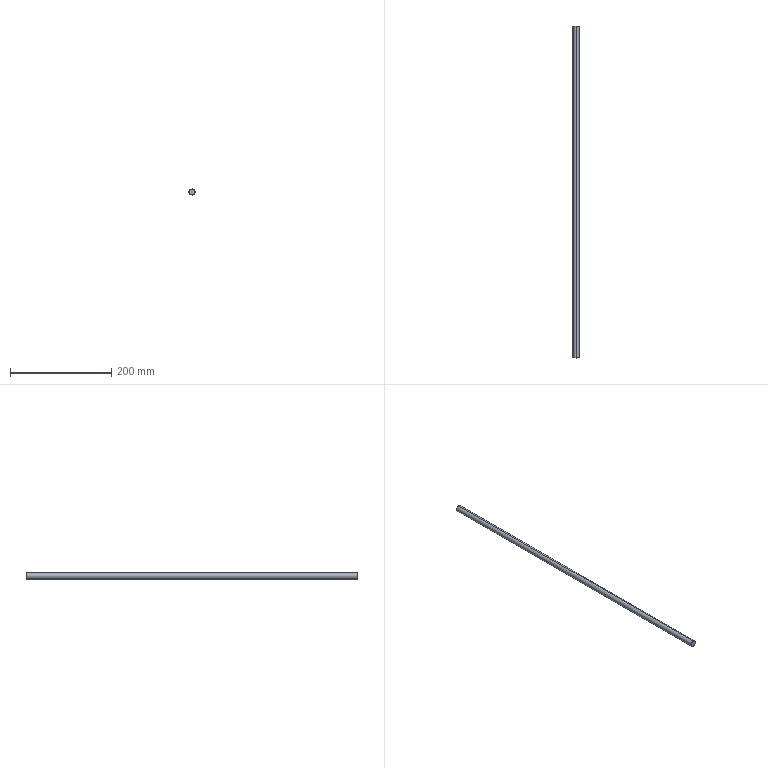Part | SolidWorks | features BaseBody 1 | 1 solid | 8 faces | box 12 x 656 x 12 mm | volume 74183 mm3 | cone 4 | cylinder 2 | plane 2 | commonest cylinder face diameters 12 x2
STEP:
#1=CARTESIAN_POINT('',(0.,0.,-5.5));
#2=VERTEX_POINT('',#1);
#3=CARTESIAN_POINT('',(0.,0.,5.5));
#4=VERTEX_POINT('',#3);
#5=CARTESIAN_POINT('',(0.,0.,0.));
#6=DIRECTION('',(0.,-1.,0.));
#7=DIRECTION('',(0.,0.,1.));
#8=AXIS2_PLACEMENT_3D('',#5,#6,#7);
#9=CIRCLE('',#8,5.5);
#10=EDGE_CURVE('',#2,#4,#9,.T.);
#11=ORIENTED_EDGE('',*,*,#10,.F.);
#12=CARTESIAN_POINT('',(0.,0.5,-6.));
#13=VERTEX_POINT('',#12);
#14=CARTESIAN_POINT('',(0.,0.5,-6.));
#15=DIRECTION('',(0.,0.7071,-0.7071));
#16=VECTOR('',#15,1000.);
#17=LINE('',#14,#16);
#18=EDGE_CURVE('',#2,#13,#17,.T.);
#19=ORIENTED_EDGE('',*,*,#18,.T.);
#20=CARTESIAN_POINT('',(0.,0.5,6.));
#21=VERTEX_POINT('',#20);
#22=CARTESIAN_POINT('',(0.,0.5,0.));
#23=DIRECTION('',(0.,1.,0.));
#24=DIRECTION('',(0.,0.,1.));
#25=AXIS2_PLACEMENT_3D('',#22,#23,#24);
#26=CIRCLE('',#25,6.);
#27=EDGE_CURVE('',#21,#13,#26,.T.);
#28=ORIENTED_EDGE('',*,*,#27,.F.);
#29=CARTESIAN_POINT('',(0.,0.5,6.));
#30=DIRECTION('',(0.,0.7071,0.7071));
#31=VECTOR('',#30,1000.);
#32=LINE('',#29,#31);
#33=EDGE_CURVE('',#4,#21,#32,.T.);
#34=ORIENTED_EDGE('',*,*,#33,.F.);
#35=EDGE_LOOP('',(#11,#19,#28,#34));
#36=FACE_OUTER_BOUND('',#35,.T.);
#37=CARTESIAN_POINT('',(0.,0.5,0.));
#38=DIRECTION('',(0.,1.,0.));
#39=DIRECTION('',(0.,0.,1.));
#40=AXIS2_PLACEMENT_3D('',#37,#38,#39);
#41=CONICAL_SURFACE('',#40,6.,0.7854);
#42=ADVANCED_FACE('',(#36),#41,.T.);
#43=CARTESIAN_POINT('',(0.,656.,5.5));
#44=VERTEX_POINT('',#43);
#45=CARTESIAN_POINT('',(0.,656.,-5.5));
#46=VERTEX_POINT('',#45);
#47=CARTESIAN_POINT('',(0.,656.,0.));
#48=DIRECTION('',(0.,1.,0.));
#49=DIRECTION('',(0.,0.,1.));
#50=AXIS2_PLACEMENT_3D('',#47,#48,#49);
#51=CIRCLE('',#50,5.5);
#52=EDGE_CURVE('',#44,#46,#51,.T.);
#53=ORIENTED_EDGE('',*,*,#52,.F.);
#54=CARTESIAN_POINT('',(0.,655.5,6.));
#55=VERTEX_POINT('',#54);
#56=CARTESIAN_POINT('',(0.,656.,5.5));
#57=DIRECTION('',(0.,-0.7071,0.7071));
#58=VECTOR('',#57,1000.);
#59=LINE('',#56,#58);
#60=EDGE_CURVE('',#44,#55,#59,.T.);
#61=ORIENTED_EDGE('',*,*,#60,.T.);
#62=CARTESIAN_POINT('',(0.,655.5,-6.));
#63=VERTEX_POINT('',#62);
#64=CARTESIAN_POINT('',(0.,655.5,0.));
#65=DIRECTION('',(0.,-1.,0.));
#66=DIRECTION('',(0.,0.,1.));
#67=AXIS2_PLACEMENT_3D('',#64,#65,#66);
#68=CIRCLE('',#67,6.);
#69=EDGE_CURVE('',#63,#55,#68,.T.);
#70=ORIENTED_EDGE('',*,*,#69,.F.);
#71=CARTESIAN_POINT('',(0.,656.,-5.5));
#72=DIRECTION('',(0.,-0.7071,-0.7071));
#73=VECTOR('',#72,1000.);
#74=LINE('',#71,#73);
#75=EDGE_CURVE('',#46,#63,#74,.T.);
#76=ORIENTED_EDGE('',*,*,#75,.F.);
#77=EDGE_LOOP('',(#53,#61,#70,#76));
#78=FACE_OUTER_BOUND('',#77,.T.);
#79=CARTESIAN_POINT('',(0.,656.,0.));
#80=DIRECTION('',(0.,-1.,0.));
#81=DIRECTION('',(0.,0.,-1.));
#82=AXIS2_PLACEMENT_3D('',#79,#80,#81);
#83=CONICAL_SURFACE('',#82,5.5,0.7854);
#84=ADVANCED_FACE('',(#78),#83,.T.);
#85=ORIENTED_EDGE('',*,*,#69,.T.);
#86=CARTESIAN_POINT('',(0.,656.,6.));
#87=DIRECTION('',(0.,-1.,0.));
#88=VECTOR('',#87,1000.);
#89=LINE('',#86,#88);
#90=EDGE_CURVE('',#55,#21,#89,.T.);
#91=ORIENTED_EDGE('',*,*,#90,.T.);
#92=ORIENTED_EDGE('',*,*,#27,.T.);
#93=CARTESIAN_POINT('',(0.,656.,-6.));
#94=DIRECTION('',(0.,-1.,0.));
#95=VECTOR('',#94,1000.);
#96=LINE('',#93,#95);
#97=EDGE_CURVE('',#63,#13,#96,.T.);
#98=ORIENTED_EDGE('',*,*,#97,.F.);
#99=EDGE_LOOP('',(#85,#91,#92,#98));
#100=FACE_OUTER_BOUND('',#99,.T.);
#101=CARTESIAN_POINT('',(0.,656.,0.));
#102=DIRECTION('',(0.,-1.,0.));
#103=DIRECTION('',(0.,0.,-1.));
#104=AXIS2_PLACEMENT_3D('',#101,#102,#103);
#105=CYLINDRICAL_SURFACE('',#104,6.);
#106=ADVANCED_FACE('',(#100),#105,.T.);
#107=CARTESIAN_POINT('',(0.,0.,0.));
#108=DIRECTION('',(0.,-1.,0.));
#109=DIRECTION('',(0.,0.,1.));
#110=AXIS2_PLACEMENT_3D('',#107,#108,#109);
#111=CIRCLE('',#110,5.5);
#112=EDGE_CURVE('',#4,#2,#111,.T.);
#113=ORIENTED_EDGE('',*,*,#112,.T.);
#114=ORIENTED_EDGE('',*,*,#10,.T.);
#115=EDGE_LOOP('',(#113,#114));
#116=FACE_OUTER_BOUND('',#115,.T.);
#117=CARTESIAN_POINT('',(0.,0.,0.));
#118=DIRECTION('',(0.,1.,0.));
#119=DIRECTION('',(1.,0.,0.));
#120=AXIS2_PLACEMENT_3D('',#117,#118,#119);
#121=PLANE('',#120);
#122=ADVANCED_FACE('',(#116),#121,.F.);
#123=CARTESIAN_POINT('',(0.,656.,0.));
#124=DIRECTION('',(0.,1.,0.));
#125=DIRECTION('',(0.,0.,1.));
#126=AXIS2_PLACEMENT_3D('',#123,#124,#125);
#127=CIRCLE('',#126,5.5);
#128=EDGE_CURVE('',#46,#44,#127,.T.);
#129=ORIENTED_EDGE('',*,*,#128,.T.);
#130=ORIENTED_EDGE('',*,*,#52,.T.);
#131=EDGE_LOOP('',(#129,#130));
#132=FACE_OUTER_BOUND('',#131,.T.);
#133=CARTESIAN_POINT('',(0.,656.,0.));
#134=DIRECTION('',(0.,1.,0.));
#135=DIRECTION('',(1.,0.,0.));
#136=AXIS2_PLACEMENT_3D('',#133,#134,#135);
#137=PLANE('',#136);
#138=ADVANCED_FACE('',(#132),#137,.T.);
#139=ORIENTED_EDGE('',*,*,#90,.F.);
#140=CARTESIAN_POINT('',(0.,655.5,0.));
#141=DIRECTION('',(0.,-1.,0.));
#142=DIRECTION('',(0.,0.,1.));
#143=AXIS2_PLACEMENT_3D('',#140,#141,#142);
#144=CIRCLE('',#143,6.);
#145=EDGE_CURVE('',#55,#63,#144,.T.);
#146=ORIENTED_EDGE('',*,*,#145,.T.);
#147=ORIENTED_EDGE('',*,*,#97,.T.);
#148=CARTESIAN_POINT('',(0.,0.5,0.));
#149=DIRECTION('',(0.,1.,0.));
#150=DIRECTION('',(0.,0.,1.));
#151=AXIS2_PLACEMENT_3D('',#148,#149,#150);
#152=CIRCLE('',#151,6.);
#153=EDGE_CURVE('',#13,#21,#152,.T.);
#154=ORIENTED_EDGE('',*,*,#153,.T.);
#155=EDGE_LOOP('',(#139,#146,#147,#154));
#156=FACE_OUTER_BOUND('',#155,.T.);
#157=CARTESIAN_POINT('',(0.,656.,0.));
#158=DIRECTION('',(0.,-1.,0.));
#159=DIRECTION('',(0.,0.,-1.));
#160=AXIS2_PLACEMENT_3D('',#157,#158,#159);
#161=CYLINDRICAL_SURFACE('',#160,6.);
#162=ADVANCED_FACE('',(#156),#161,.T.);
#163=ORIENTED_EDGE('',*,*,#60,.F.);
#164=ORIENTED_EDGE('',*,*,#128,.F.);
#165=ORIENTED_EDGE('',*,*,#75,.T.);
#166=ORIENTED_EDGE('',*,*,#145,.F.);
#167=EDGE_LOOP('',(#163,#164,#165,#166));
#168=FACE_OUTER_BOUND('',#167,.T.);
#169=CARTESIAN_POINT('',(0.,656.,0.));
#170=DIRECTION('',(0.,-1.,0.));
#171=DIRECTION('',(0.,0.,-1.));
#172=AXIS2_PLACEMENT_3D('',#169,#170,#171);
#173=CONICAL_SURFACE('',#172,5.5,0.7854);
#174=ADVANCED_FACE('',(#168),#173,.T.);
#175=ORIENTED_EDGE('',*,*,#18,.F.);
#176=ORIENTED_EDGE('',*,*,#112,.F.);
#177=ORIENTED_EDGE('',*,*,#33,.T.);
#178=ORIENTED_EDGE('',*,*,#153,.F.);
#179=EDGE_LOOP('',(#175,#176,#177,#178));
#180=FACE_OUTER_BOUND('',#179,.T.);
#181=CARTESIAN_POINT('',(0.,0.5,0.));
#182=DIRECTION('',(0.,1.,0.));
#183=DIRECTION('',(0.,0.,1.));
#184=AXIS2_PLACEMENT_3D('',#181,#182,#183);
#185=CONICAL_SURFACE('',#184,6.,0.7854);
#186=ADVANCED_FACE('',(#180),#185,.T.);
#187=CLOSED_SHELL('',(#42,#84,#106,#122,#138,#162,#174,#186));
#188=MANIFOLD_SOLID_BREP('',#187);
#189=CARTESIAN_POINT('',(0.,0.,0.));
#190=DIRECTION('',(0.,0.,1.));
#191=DIRECTION('',(1.,0.,0.));
#192=AXIS2_PLACEMENT_3D('',#189,#190,#191);
#193=(LENGTH_UNIT()NAMED_UNIT(*)SI_UNIT(.MILLI.,.METRE.));
#194=UNCERTAINTY_MEASURE_WITH_UNIT(LENGTH_MEASURE(0.00001),#193,'','');
#195=(NAMED_UNIT(*)PLANE_ANGLE_UNIT()SI_UNIT($,.RADIAN.));
#196=(NAMED_UNIT(*)SI_UNIT($,.STERADIAN.)SOLID_ANGLE_UNIT());
#197=(GEOMETRIC_REPRESENTATION_CONTEXT(3)GLOBAL_UNCERTAINTY_ASSIGNED_CONTEXT((#194))GLOBAL_UNIT_ASSIGNED_CONTEXT((#193,#195,#196))REPRESENTATION_CONTEXT('',''));
#198=ADVANCED_BREP_SHAPE_REPRESENTATION('',(#188,#192),#197);